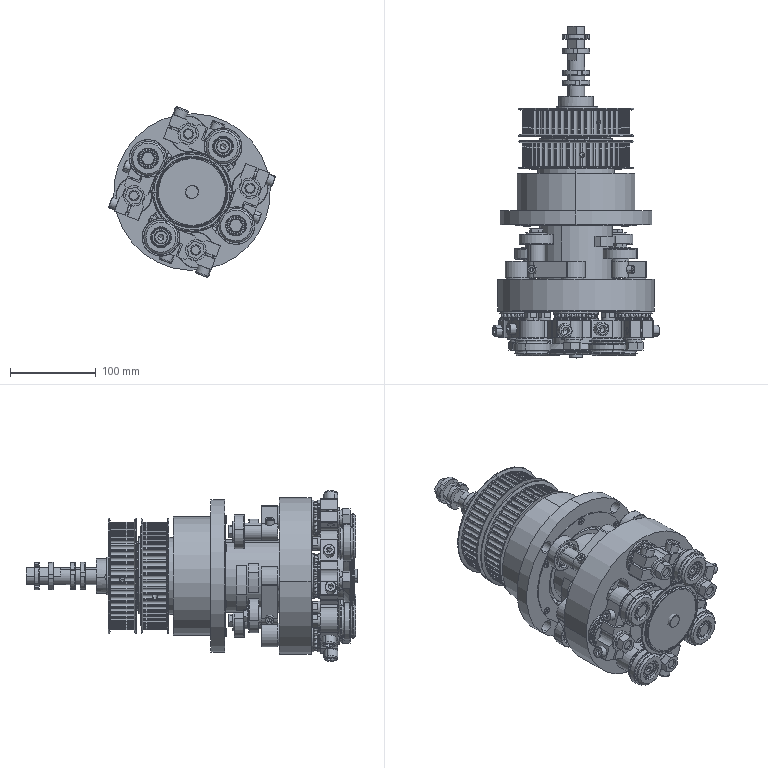Part | SolidWorks | 159 solids | 12166 faces | volume 3128035 mm3 | spline 6413 | cylinder 3193 | plane 2274 | cone 286 | commonest cylinder face diameters 0.75 x860 16.285 x380 0.81 x254 5.184 x150 125.95 x104 29 x80